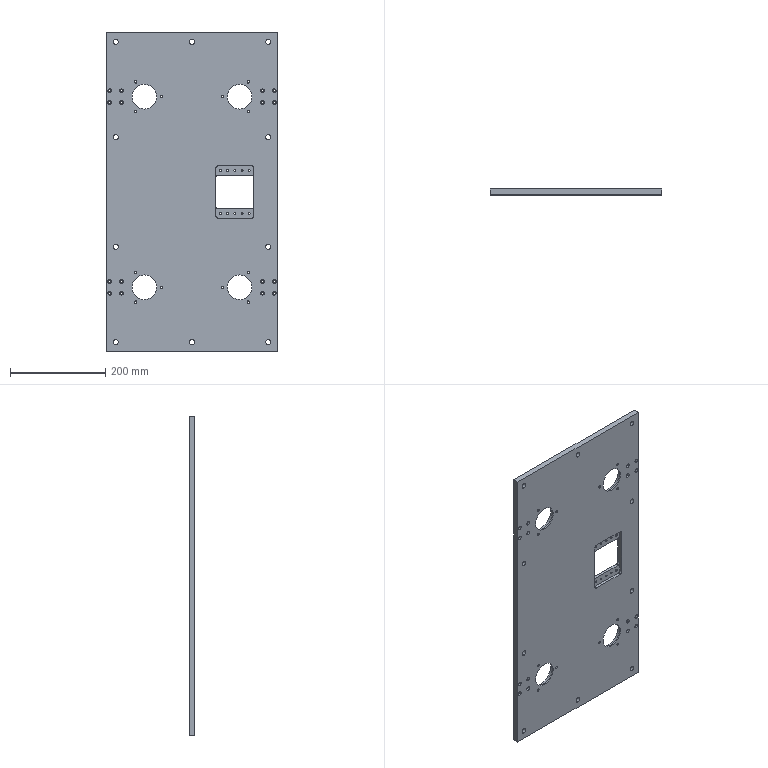Part | SolidWorks | features ICE 5, HoleWzd 3, Extrusion 1 | 1 solid | 186 faces | box 359 x 12 x 668 mm | volume 2636785 mm3 | cylinder 152 | plane 34 | commonest cylinder face diameters 4.5 x32 8 x32 5 x24 4.2 x20 11 x20 10 x8